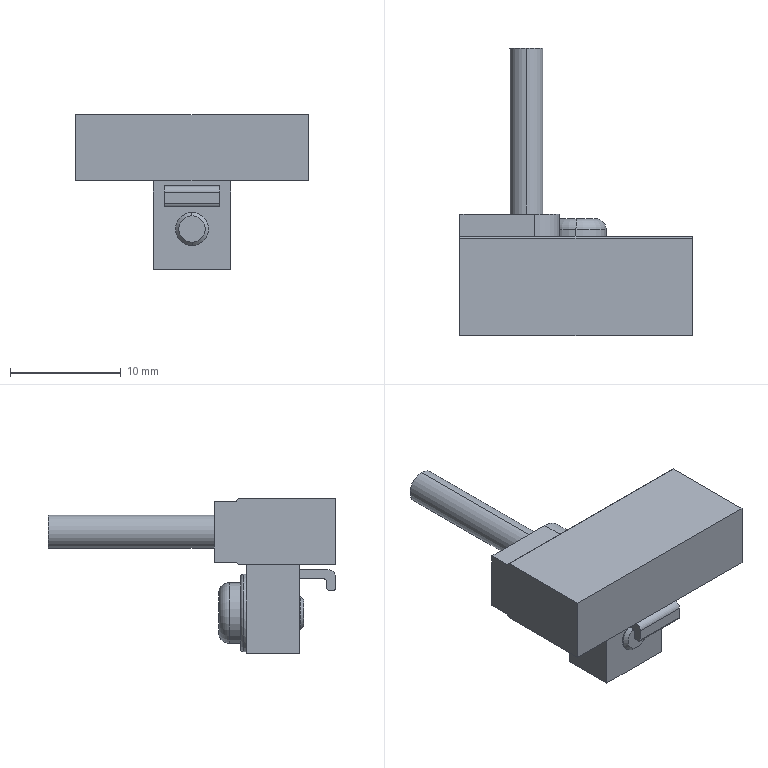Part | SolidWorks | features BaseBody 1 | 1 solid | 49 faces | box 21 x 26 x 14 mm | volume 1685 mm3 | plane 29 | cylinder 14 | torus 4 | cone 2 | commonest cylinder face diameters 3 x4 0.5 x2 4.5 x2 5.5 x2 7 x2 0.6 x1
STEP:
#1=CARTESIAN_POINT('',(10.5,9.6,-4.6));
#2=VERTEX_POINT('',#1);
#3=CARTESIAN_POINT('',(10.5,10.6,-5.6));
#4=VERTEX_POINT('',#3);
#5=CARTESIAN_POINT('',(10.5,9.6,-5.6));
#6=DIRECTION('',(-1.,0.,0.));
#7=DIRECTION('',(0.,0.,1.));
#8=AXIS2_PLACEMENT_3D('',#5,#6,#7);
#9=CIRCLE('',#8,1.);
#10=EDGE_CURVE('',#2,#4,#9,.T.);
#11=ORIENTED_EDGE('',*,*,#10,.F.);
#12=CARTESIAN_POINT('',(10.5,9.6,-10.1));
#13=VERTEX_POINT('',#12);
#14=CARTESIAN_POINT('',(10.5,9.6,-7.35));
#15=DIRECTION('',(0.,1.,0.));
#16=DIRECTION('',(0.,0.,1.));
#17=AXIS2_PLACEMENT_3D('',#14,#15,#16);
#18=CIRCLE('',#17,2.75);
#19=EDGE_CURVE('',#2,#13,#18,.T.);
#20=ORIENTED_EDGE('',*,*,#19,.T.);
#21=CARTESIAN_POINT('',(10.5,10.6,-9.1));
#22=VERTEX_POINT('',#21);
#23=CARTESIAN_POINT('',(10.5,9.6,-9.1));
#24=DIRECTION('',(1.,0.,0.));
#25=DIRECTION('',(0.,0.,-1.));
#26=AXIS2_PLACEMENT_3D('',#23,#24,#25);
#27=CIRCLE('',#26,1.);
#28=EDGE_CURVE('',#13,#22,#27,.T.);
#29=ORIENTED_EDGE('',*,*,#28,.T.);
#30=CARTESIAN_POINT('',(10.5,10.6,-7.35));
#31=DIRECTION('',(0.,1.,0.));
#32=DIRECTION('',(0.,0.,-1.));
#33=AXIS2_PLACEMENT_3D('',#30,#31,#32);
#34=CIRCLE('',#33,1.75);
#35=EDGE_CURVE('',#4,#22,#34,.T.);
#36=ORIENTED_EDGE('',*,*,#35,.F.);
#37=EDGE_LOOP('',(#11,#20,#29,#36));
#38=FACE_OUTER_BOUND('',#37,.T.);
#39=CARTESIAN_POINT('',(10.5,9.6,-7.35));
#40=DIRECTION('',(0.,1.,0.));
#41=DIRECTION('',(0.,0.,-1.));
#42=AXIS2_PLACEMENT_3D('',#39,#40,#41);
#43=TOROIDAL_SURFACE('',#42,1.75,1.);
#44=ADVANCED_FACE('',(#38),#43,.T.);
#45=CARTESIAN_POINT('',(10.5,8.6,-4.6));
#46=VERTEX_POINT('',#45);
#47=CARTESIAN_POINT('',(10.5,10.6,-4.6));
#48=DIRECTION('',(0.,1.,0.));
#49=VECTOR('',#48,1000.);
#50=LINE('',#47,#49);
#51=EDGE_CURVE('',#46,#2,#50,.T.);
#52=ORIENTED_EDGE('',*,*,#51,.F.);
#53=CARTESIAN_POINT('',(10.5,8.6,-10.1));
#54=VERTEX_POINT('',#53);
#55=CARTESIAN_POINT('',(10.5,8.6,-7.35));
#56=DIRECTION('',(0.,1.,0.));
#57=DIRECTION('',(0.,0.,1.));
#58=AXIS2_PLACEMENT_3D('',#55,#56,#57);
#59=CIRCLE('',#58,2.75);
#60=EDGE_CURVE('',#46,#54,#59,.T.);
#61=ORIENTED_EDGE('',*,*,#60,.T.);
#62=CARTESIAN_POINT('',(10.5,10.6,-10.1));
#63=DIRECTION('',(0.,1.,0.));
#64=VECTOR('',#63,1000.);
#65=LINE('',#62,#64);
#66=EDGE_CURVE('',#54,#13,#65,.T.);
#67=ORIENTED_EDGE('',*,*,#66,.T.);
#68=ORIENTED_EDGE('',*,*,#19,.F.);
#69=EDGE_LOOP('',(#52,#61,#67,#68));
#70=FACE_OUTER_BOUND('',#69,.T.);
#71=CARTESIAN_POINT('',(10.5,10.6,-7.35));
#72=DIRECTION('',(0.,1.,0.));
#73=DIRECTION('',(0.000000142,0.,-1.));
#74=AXIS2_PLACEMENT_3D('',#71,#72,#73);
#75=CYLINDRICAL_SURFACE('',#74,2.75);
#76=ADVANCED_FACE('',(#70),#75,.T.);
#77=CARTESIAN_POINT('',(10.5,8.35,-3.85));
#78=VERTEX_POINT('',#77);
#79=CARTESIAN_POINT('',(10.5,8.6,-4.1));
#80=VERTEX_POINT('',#79);
#81=CARTESIAN_POINT('',(10.5,8.35,-4.1));
#82=DIRECTION('',(-1.,0.,-0.000000141));
#83=DIRECTION('',(-0.000000141,0.,1.));
#84=AXIS2_PLACEMENT_3D('',#81,#82,#83);
#85=CIRCLE('',#84,0.25);
#86=EDGE_CURVE('',#78,#80,#85,.T.);
#87=ORIENTED_EDGE('',*,*,#86,.F.);
#88=CARTESIAN_POINT('',(10.5,8.35,-10.85));
#89=VERTEX_POINT('',#88);
#90=CARTESIAN_POINT('',(10.5,8.35,-7.35));
#91=DIRECTION('',(0.,1.,0.));
#92=DIRECTION('',(0.,0.,1.));
#93=AXIS2_PLACEMENT_3D('',#90,#91,#92);
#94=CIRCLE('',#93,3.5);
#95=EDGE_CURVE('',#78,#89,#94,.T.);
#96=ORIENTED_EDGE('',*,*,#95,.T.);
#97=CARTESIAN_POINT('',(10.5,8.6,-10.6));
#98=VERTEX_POINT('',#97);
#99=CARTESIAN_POINT('',(10.5,8.35,-10.6));
#100=DIRECTION('',(1.,0.,0.000000141));
#101=DIRECTION('',(0.000000141,0.,-1.));
#102=AXIS2_PLACEMENT_3D('',#99,#100,#101);
#103=CIRCLE('',#102,0.25);
#104=EDGE_CURVE('',#89,#98,#103,.T.);
#105=ORIENTED_EDGE('',*,*,#104,.T.);
#106=CARTESIAN_POINT('',(10.5,8.6,-7.35));
#107=DIRECTION('',(0.,1.,0.));
#108=DIRECTION('',(0.000000141,0.,-1.));
#109=AXIS2_PLACEMENT_3D('',#106,#107,#108);
#110=CIRCLE('',#109,3.25);
#111=EDGE_CURVE('',#80,#98,#110,.T.);
#112=ORIENTED_EDGE('',*,*,#111,.F.);
#113=EDGE_LOOP('',(#87,#96,#105,#112));
#114=FACE_OUTER_BOUND('',#113,.T.);
#115=CARTESIAN_POINT('',(10.5,8.35,-7.35));
#116=DIRECTION('',(0.,1.,0.));
#117=DIRECTION('',(0.000000141,0.,-1.));
#118=AXIS2_PLACEMENT_3D('',#115,#116,#117);
#119=TOROIDAL_SURFACE('',#118,3.25,0.25);
#120=ADVANCED_FACE('',(#114),#119,.T.);
#121=CARTESIAN_POINT('',(10.5,8.1,-3.85));
#122=VERTEX_POINT('',#121);
#123=CARTESIAN_POINT('',(10.5,10.6,-3.85));
#124=DIRECTION('',(0.,1.,0.));
#125=VECTOR('',#124,1000.);
#126=LINE('',#123,#125);
#127=EDGE_CURVE('',#122,#78,#126,.T.);
#128=ORIENTED_EDGE('',*,*,#127,.F.);
#129=CARTESIAN_POINT('',(14.,8.1,-7.35));
#130=VERTEX_POINT('',#129);
#131=CARTESIAN_POINT('',(10.5,8.1,-7.35));
#132=DIRECTION('',(0.,1.,0.));
#133=DIRECTION('',(0.,0.,1.));
#134=AXIS2_PLACEMENT_3D('',#131,#132,#133);
#135=CIRCLE('',#134,3.5);
#136=EDGE_CURVE('',#122,#130,#135,.T.);
#137=ORIENTED_EDGE('',*,*,#136,.T.);
#138=CARTESIAN_POINT('',(10.5,8.1,-10.85));
#139=VERTEX_POINT('',#138);
#140=CARTESIAN_POINT('',(10.5,8.1,-7.35));
#141=DIRECTION('',(0.,1.,0.));
#142=DIRECTION('',(0.,0.,-1.));
#143=AXIS2_PLACEMENT_3D('',#140,#141,#142);
#144=CIRCLE('',#143,3.5);
#145=EDGE_CURVE('',#130,#139,#144,.T.);
#146=ORIENTED_EDGE('',*,*,#145,.T.);
#147=CARTESIAN_POINT('',(10.5,10.6,-10.85));
#148=DIRECTION('',(0.,1.,0.));
#149=VECTOR('',#148,1000.);
#150=LINE('',#147,#149);
#151=EDGE_CURVE('',#139,#89,#150,.T.);
#152=ORIENTED_EDGE('',*,*,#151,.T.);
#153=ORIENTED_EDGE('',*,*,#95,.F.);
#154=EDGE_LOOP('',(#128,#137,#146,#152,#153));
#155=FACE_OUTER_BOUND('',#154,.T.);
#156=CARTESIAN_POINT('',(10.5,10.6,-7.35));
#157=DIRECTION('',(0.,1.,0.));
#158=DIRECTION('',(0.,0.,-1.));
#159=AXIS2_PLACEMENT_3D('',#156,#157,#158);
#160=CYLINDRICAL_SURFACE('',#159,3.5);
#161=ADVANCED_FACE('',(#155),#160,.T.);
#162=CARTESIAN_POINT('',(10.5,3.207,-5.85));
#163=VERTEX_POINT('',#162);
#164=CARTESIAN_POINT('',(10.5,3.3,-5.85));
#165=VERTEX_POINT('',#164);
#166=CARTESIAN_POINT('',(10.5,10.6,-5.85));
#167=DIRECTION('',(0.,1.,0.));
#168=VECTOR('',#167,1000.);
#169=LINE('',#166,#168);
#170=EDGE_CURVE('',#163,#165,#169,.T.);
#171=ORIENTED_EDGE('',*,*,#170,.F.);
#172=CARTESIAN_POINT('',(10.5,3.207,-8.85));
#173=VERTEX_POINT('',#172);
#174=CARTESIAN_POINT('',(10.5,3.207,-7.35));
#175=DIRECTION('',(0.,1.,0.));
#176=DIRECTION('',(0.,0.,1.));
#177=AXIS2_PLACEMENT_3D('',#174,#175,#176);
#178=CIRCLE('',#177,1.5);
#179=EDGE_CURVE('',#163,#173,#178,.T.);
#180=ORIENTED_EDGE('',*,*,#179,.T.);
#181=CARTESIAN_POINT('',(10.5,3.3,-8.85));
#182=VERTEX_POINT('',#181);
#183=CARTESIAN_POINT('',(10.5,10.6,-8.85));
#184=DIRECTION('',(0.,1.,0.));
#185=VECTOR('',#184,1000.);
#186=LINE('',#183,#185);
#187=EDGE_CURVE('',#173,#182,#186,.T.);
#188=ORIENTED_EDGE('',*,*,#187,.T.);
#189=CARTESIAN_POINT('',(10.5,3.3,-7.35));
#190=DIRECTION('',(0.,-1.,0.));
#191=DIRECTION('',(-0.000000142,0.,-1.));
#192=AXIS2_PLACEMENT_3D('',#189,#190,#191);
#193=CIRCLE('',#192,1.5);
#194=EDGE_CURVE('',#182,#165,#193,.T.);
#195=ORIENTED_EDGE('',*,*,#194,.T.);
#196=EDGE_LOOP('',(#171,#180,#188,#195));
#197=FACE_OUTER_BOUND('',#196,.T.);
#198=CARTESIAN_POINT('',(10.5,10.6,-7.35));
#199=DIRECTION('',(0.,1.,0.));
#200=DIRECTION('',(0.,0.,-1.));
#201=AXIS2_PLACEMENT_3D('',#198,#199,#200);
#202=CYLINDRICAL_SURFACE('',#201,1.5);
#203=ADVANCED_FACE('',(#197),#202,.T.);
#204=CARTESIAN_POINT('',(10.5,2.9,-6.156));
#205=VERTEX_POINT('',#204);
#206=CARTESIAN_POINT('',(10.5,3.207,-5.85));
#207=DIRECTION('',(-0.000000101,0.7071,0.7071));
#208=VECTOR('',#207,1000.);
#209=LINE('',#206,#208);
#210=EDGE_CURVE('',#205,#163,#209,.T.);
#211=ORIENTED_EDGE('',*,*,#210,.F.);
#212=CARTESIAN_POINT('',(10.5,2.9,-8.543));
#213=VERTEX_POINT('',#212);
#214=CARTESIAN_POINT('',(10.5,2.9,-7.35));
#215=DIRECTION('',(0.,1.,0.));
#216=DIRECTION('',(0.,0.,1.));
#217=AXIS2_PLACEMENT_3D('',#214,#215,#216);
#218=CIRCLE('',#217,1.194);
#219=EDGE_CURVE('',#205,#213,#218,.T.);
#220=ORIENTED_EDGE('',*,*,#219,.T.);
#221=CARTESIAN_POINT('',(10.5,3.207,-8.85));
#222=DIRECTION('',(0.000000101,0.7071,-0.7071));
#223=VECTOR('',#222,1000.);
#224=LINE('',#221,#223);
#225=EDGE_CURVE('',#213,#173,#224,.T.);
#226=ORIENTED_EDGE('',*,*,#225,.T.);
#227=ORIENTED_EDGE('',*,*,#179,.F.);
#228=EDGE_LOOP('',(#211,#220,#226,#227));
#229=FACE_OUTER_BOUND('',#228,.T.);
#230=CARTESIAN_POINT('',(10.5,3.207,-7.35));
#231=DIRECTION('',(0.,1.,0.));
#232=DIRECTION('',(0.000000142,0.,-1.));
#233=AXIS2_PLACEMENT_3D('',#230,#231,#232);
#234=CONICAL_SURFACE('',#233,1.5,0.7854);
#235=ADVANCED_FACE('',(#229),#234,.T.);
#236=CARTESIAN_POINT('',(6.,11.,1.5));
#237=VERTEX_POINT('',#236);
#238=CARTESIAN_POINT('',(6.,26.,1.5));
#239=VERTEX_POINT('',#238);
#240=CARTESIAN_POINT('',(6.,26.,1.5));
#241=DIRECTION('',(0.,1.,0.));
#242=VECTOR('',#241,1000.);
#243=LINE('',#240,#242);
#244=EDGE_CURVE('',#237,#239,#243,.T.);
#245=ORIENTED_EDGE('',*,*,#244,.F.);
#246=CARTESIAN_POINT('',(6.,11.,-1.5));
#247=VERTEX_POINT('',#246);
#248=CARTESIAN_POINT('',(6.,11.,0.));
#249=DIRECTION('',(0.,1.,0.));
#250=DIRECTION('',(0.,0.,1.));
#251=AXIS2_PLACEMENT_3D('',#248,#249,#250);
#252=CIRCLE('',#251,1.5);
#253=EDGE_CURVE('',#237,#247,#252,.T.);
#254=ORIENTED_EDGE('',*,*,#253,.T.);
#255=CARTESIAN_POINT('',(6.,26.,-1.5));
#256=VERTEX_POINT('',#255);
#257=CARTESIAN_POINT('',(6.,26.,-1.5));
#258=DIRECTION('',(0.,1.,0.));
#259=VECTOR('',#258,1000.);
#260=LINE('',#257,#259);
#261=EDGE_CURVE('',#247,#256,#260,.T.);
#262=ORIENTED_EDGE('',*,*,#261,.T.);
#263=CARTESIAN_POINT('',(6.,26.,0.));
#264=DIRECTION('',(0.,1.,0.));
#265=DIRECTION('',(0.,0.,-1.));
#266=AXIS2_PLACEMENT_3D('',#263,#264,#265);
#267=CIRCLE('',#266,1.5);
#268=EDGE_CURVE('',#239,#256,#267,.T.);
#269=ORIENTED_EDGE('',*,*,#268,.F.);
#270=EDGE_LOOP('',(#245,#254,#262,#269));
#271=FACE_OUTER_BOUND('',#270,.T.);
#272=CARTESIAN_POINT('',(6.,26.,0.));
#273=DIRECTION('',(0.,1.,0.));
#274=DIRECTION('',(0.,0.,-1.));
#275=AXIS2_PLACEMENT_3D('',#272,#273,#274);
#276=CYLINDRICAL_SURFACE('',#275,1.5);
#277=ADVANCED_FACE('',(#271),#276,.T.);
#278=CARTESIAN_POINT('',(10.5,10.6,-7.35));
#279=DIRECTION('',(0.,1.,0.));
#280=DIRECTION('',(0.,0.,-1.));
#281=AXIS2_PLACEMENT_3D('',#278,#279,#280);
#282=CIRCLE('',#281,1.75);
#283=EDGE_CURVE('',#22,#4,#282,.T.);
#284=ORIENTED_EDGE('',*,*,#283,.T.);
#285=ORIENTED_EDGE('',*,*,#35,.T.);
#286=EDGE_LOOP('',(#284,#285));
#287=FACE_OUTER_BOUND('',#286,.T.);
#288=CARTESIAN_POINT('',(8.75,10.6,-5.6));
#289=DIRECTION('',(0.,1.,0.));
#290=DIRECTION('',(1.,0.,0.));
#291=AXIS2_PLACEMENT_3D('',#288,#289,#290);
#292=PLANE('',#291);
#293=ADVANCED_FACE('',(#287),#292,.T.);
#294=CARTESIAN_POINT('',(10.5,8.6,-7.35));
#295=DIRECTION('',(0.,1.,0.));
#296=DIRECTION('',(0.,0.,1.));
#297=AXIS2_PLACEMENT_3D('',#294,#295,#296);
#298=CIRCLE('',#297,2.75);
#299=EDGE_CURVE('',#54,#46,#298,.T.);
#300=ORIENTED_EDGE('',*,*,#299,.F.);
#301=ORIENTED_EDGE('',*,*,#60,.F.);
#302=EDGE_LOOP('',(#300,#301));
#303=FACE_BOUND('',#302,.T.);
#304=CARTESIAN_POINT('',(10.5,8.6,-7.35));
#305=DIRECTION('',(0.,1.,0.));
#306=DIRECTION('',(0.000000141,0.,-1.));
#307=AXIS2_PLACEMENT_3D('',#304,#305,#306);
#308=CIRCLE('',#307,3.25);
#309=EDGE_CURVE('',#98,#80,#308,.T.);
#310=ORIENTED_EDGE('',*,*,#309,.T.);
#311=ORIENTED_EDGE('',*,*,#111,.T.);
#312=EDGE_LOOP('',(#310,#311));
#313=FACE_OUTER_BOUND('',#312,.T.);
#314=CARTESIAN_POINT('',(7.25,8.6,-4.1));
#315=DIRECTION('',(0.,1.,0.));
#316=DIRECTION('',(1.,0.,0.));
#317=AXIS2_PLACEMENT_3D('',#314,#315,#316);
#318=PLANE('',#317);
#319=ADVANCED_FACE('',(#303,#313),#318,.T.);
#320=CARTESIAN_POINT('',(10.5,2.9,-7.35));
#321=DIRECTION('',(0.,1.,0.));
#322=DIRECTION('',(0.,0.,1.));
#323=AXIS2_PLACEMENT_3D('',#320,#321,#322);
#324=CIRCLE('',#323,1.194);
#325=EDGE_CURVE('',#213,#205,#324,.T.);
#326=ORIENTED_EDGE('',*,*,#325,.F.);
#327=ORIENTED_EDGE('',*,*,#219,.F.);
#328=EDGE_LOOP('',(#326,#327));
#329=FACE_OUTER_BOUND('',#328,.T.);
#330=CARTESIAN_POINT('',(9.291,2.9,-8.544));
#331=DIRECTION('',(0.,-1.,0.));
#332=DIRECTION('',(0.,0.,-1.));
#333=AXIS2_PLACEMENT_3D('',#330,#331,#332);
#334=PLANE('',#333);
#335=ADVANCED_FACE('',(#329),#334,.T.);
#336=CARTESIAN_POINT('',(8.,1.1,-4.25));
#337=VERTEX_POINT('',#336);
#338=CARTESIAN_POINT('',(8.,0.8,-4.55));
#339=VERTEX_POINT('',#338);
#340=CARTESIAN_POINT('',(8.,1.1,-4.55));
#341=DIRECTION('',(1.,0.,0.));
#342=DIRECTION('',(0.,0.,1.));
#343=AXIS2_PLACEMENT_3D('',#340,#341,#342);
#344=CIRCLE('',#343,0.3);
#345=EDGE_CURVE('',#337,#339,#344,.T.);
#346=ORIENTED_EDGE('',*,*,#345,.F.);
#347=CARTESIAN_POINT('',(13.,1.1,-4.25));
#348=VERTEX_POINT('',#347);
#349=CARTESIAN_POINT('',(13.,1.1,-4.25));
#350=DIRECTION('',(-1.,0.,0.));
#351=VECTOR('',#350,1000.);
#352=LINE('',#349,#351);
#353=EDGE_CURVE('',#348,#337,#352,.T.);
#354=ORIENTED_EDGE('',*,*,#353,.F.);
#355=CARTESIAN_POINT('',(13.,0.8,-4.55));
#356=VERTEX_POINT('',#355);
#357=CARTESIAN_POINT('',(13.,1.1,-4.55));
#358=DIRECTION('',(1.,0.,0.));
#359=DIRECTION('',(0.,-1.,0.));
#360=AXIS2_PLACEMENT_3D('',#357,#358,#359);
#361=CIRCLE('',#360,0.3);
#362=EDGE_CURVE('',#348,#356,#361,.T.);
#363=ORIENTED_EDGE('',*,*,#362,.T.);
#364=CARTESIAN_POINT('',(8.,0.8,-4.55));
#365=DIRECTION('',(-1.,0.,0.));
#366=VECTOR('',#365,1000.);
#367=LINE('',#364,#366);
#368=EDGE_CURVE('',#356,#339,#367,.T.);
#369=ORIENTED_EDGE('',*,*,#368,.T.);
#370=EDGE_LOOP('',(#346,#354,#363,#369));
#371=FACE_OUTER_BOUND('',#370,.T.);
#372=CARTESIAN_POINT('',(13.,1.1,-4.55));
#373=DIRECTION('',(-1.,0.,0.));
#374=DIRECTION('',(0.,-1.,0.));
#375=AXIS2_PLACEMENT_3D('',#372,#373,#374);
#376=CYLINDRICAL_SURFACE('',#375,0.3);
#377=ADVANCED_FACE('',(#371),#376,.F.);
#378=CARTESIAN_POINT('',(8.,0.8,-5.07));
#379=VERTEX_POINT('',#378);
#380=CARTESIAN_POINT('',(8.,0.8,-4.55));
#381=DIRECTION('',(0.,0.,1.));
#382=VECTOR('',#381,1000.);
#383=LINE('',#380,#382);
#384=EDGE_CURVE('',#379,#339,#383,.T.);
#385=ORIENTED_EDGE('',*,*,#384,.T.);
#386=ORIENTED_EDGE('',*,*,#368,.F.);
#387=CARTESIAN_POINT('',(13.,0.8,-5.07));
#388=VERTEX_POINT('',#387);
#389=CARTESIAN_POINT('',(13.,0.8,-5.07));
#390=DIRECTION('',(0.,0.,1.));
#391=VECTOR('',#390,1000.);
#392=LINE('',#389,#391);
#393=EDGE_CURVE('',#388,#356,#392,.T.);
#394=ORIENTED_EDGE('',*,*,#393,.F.);
#395=CARTESIAN_POINT('',(8.,0.8,-5.07));
#396=DIRECTION('',(-1.,0.,0.));
#397=VECTOR('',#396,1000.);
#398=LINE('',#395,#397);
#399=EDGE_CURVE('',#388,#379,#398,.T.);
#400=ORIENTED_EDGE('',*,*,#399,.T.);
#401=EDGE_LOOP('',(#385,#386,#394,#400));
#402=FACE_OUTER_BOUND('',#401,.T.);
#403=CARTESIAN_POINT('',(8.,0.8,-4.55));
#404=DIRECTION('',(0.,1.,0.));
#405=DIRECTION('',(1.,0.,0.));
#406=AXIS2_PLACEMENT_3D('',#403,#404,#405);
#407=PLANE('',#406);
#408=ADVANCED_FACE('',(#402),#407,.T.);
#409=CARTESIAN_POINT('',(8.,0.55,-5.32));
#410=VERTEX_POINT('',#409);
#411=CARTESIAN_POINT('',(8.,0.55,-5.07));
#412=DIRECTION('',(1.,0.,0.));
#413=DIRECTION('',(0.,1.,0.));
#414=AXIS2_PLACEMENT_3D('',#411,#412,#413);
#415=CIRCLE('',#414,0.25);
#416=EDGE_CURVE('',#410,#379,#415,.T.);
#417=ORIENTED_EDGE('',*,*,#416,.T.);
#418=ORIENTED_EDGE('',*,*,#399,.F.);
#419=CARTESIAN_POINT('',(13.,0.55,-5.32));
#420=VERTEX_POINT('',#419);
#421=CARTESIAN_POINT('',(13.,0.55,-5.07));
#422=DIRECTION('',(1.,0.,0.));
#423=DIRECTION('',(0.,0.,-1.));
#424=AXIS2_PLACEMENT_3D('',#421,#422,#423);
#425=CIRCLE('',#424,0.25);
#426=EDGE_CURVE('',#420,#388,#425,.T.);
#427=ORIENTED_EDGE('',*,*,#426,.F.);
#428=CARTESIAN_POINT('',(8.,0.55,-5.32));
#429=DIRECTION('',(-1.,0.,0.));
#430=VECTOR('',#429,1000.);
#431=LINE('',#428,#430);
#432=EDGE_CURVE('',#420,#410,#431,.T.);
#433=ORIENTED_EDGE('',*,*,#432,.T.);
#434=EDGE_LOOP('',(#417,#418,#427,#433));
#435=FACE_OUTER_BOUND('',#434,.T.);
#436=CARTESIAN_POINT('',(13.,0.55,-5.07));
#437=DIRECTION('',(-1.,0.,0.));
#438=DIRECTION('',(0.,1.,0.));
#439=AXIS2_PLACEMENT_3D('',#436,#437,#438);
#440=CYLINDRICAL_SURFACE('',#439,0.25);
#441=ADVANCED_FACE('',(#435),#440,.T.);
#442=CARTESIAN_POINT('',(8.,0.25,-5.32));
#443=VERTEX_POINT('',#442);
#444=CARTESIAN_POINT('',(8.,0.55,-5.32));
#445=DIRECTION('',(0.,1.,0.));
#446=VECTOR('',#445,1000.);
#447=LINE('',#444,#446);
#448=EDGE_CURVE('',#443,#410,#447,.T.);
#449=ORIENTED_EDGE('',*,*,#448,.T.);
#450=ORIENTED_EDGE('',*,*,#432,.F.);
#451=CARTESIAN_POINT('',(13.,0.25,-5.32));
#452=VERTEX_POINT('',#451);
#453=CARTESIAN_POINT('',(13.,0.25,-5.32));
#454=DIRECTION('',(0.,1.,0.));
#455=VECTOR('',#454,1000.);
#456=LINE('',#453,#455);
#457=EDGE_CURVE('',#452,#420,#456,.T.);
#458=ORIENTED_EDGE('',*,*,#457,.F.);
#459=CARTESIAN_POINT('',(8.,0.25,-5.32));
#460=DIRECTION('',(-1.,0.,0.));
#461=VECTOR('',#460,1000.);
#462=LINE('',#459,#461);
#463=EDGE_CURVE('',#452,#443,#462,.T.);
#464=ORIENTED_EDGE('',*,*,#463,.T.);
#465=EDGE_LOOP('',(#449,#450,#458,#464));
#466=FACE_OUTER_BOUND('',#465,.T.);
#467=CARTESIAN_POINT('',(8.,0.25,-5.32));
#468=DIRECTION('',(0.,0.,-1.));
#469=DIRECTION('',(0.,-1.,0.));
#470=AXIS2_PLACEMENT_3D('',#467,#468,#469);
#471=PLANE('',#470);
#472=ADVANCED_FACE('',(#466),#471,.T.);
#473=CARTESIAN_POINT('',(8.,0.,-5.07));
#474=VERTEX_POINT('',#473);
#475=CARTESIAN_POINT('',(8.,0.25,-5.07));
#476=DIRECTION('',(1.,0.,0.));
#477=DIRECTION('',(0.,0.,-1.));
#478=AXIS2_PLACEMENT_3D('',#475,#476,#477);
#479=CIRCLE('',#478,0.25);
#480=EDGE_CURVE('',#474,#443,#479,.T.);
#481=ORIENTED_EDGE('',*,*,#480,.T.);
#482=ORIENTED_EDGE('',*,*,#463,.F.);
#483=CARTESIAN_POINT('',(13.,0.,-5.07));
#484=VERTEX_POINT('',#483);
#485=CARTESIAN_POINT('',(13.,0.25,-5.07));
#486=DIRECTION('',(1.,0.,0.));
#487=DIRECTION('',(0.,-1.,0.));
#488=AXIS2_PLACEMENT_3D('',#485,#486,#487);
#489=CIRCLE('',#488,0.25);
#490=EDGE_CURVE('',#484,#452,#489,.T.);
#491=ORIENTED_EDGE('',*,*,#490,.F.);
#492=CARTESIAN_POINT('',(8.,0.,-5.07));
#493=DIRECTION('',(-1.,0.,0.));
#494=VECTOR('',#493,1000.);
#495=LINE('',#492,#494);
#496=EDGE_CURVE('',#484,#474,#495,.T.);
#497=ORIENTED_EDGE('',*,*,#496,.T.);
#498=EDGE_LOOP('',(#481,#482,#491,#497));
#499=FACE_OUTER_BOUND('',#498,.T.);
#500=CARTESIAN_POINT('',(13.,0.25,-5.07));
#501=DIRECTION('',(-1.,0.,0.));
#502=DIRECTION('',(0.,0.,-1.));
#503=AXIS2_PLACEMENT_3D('',#500,#501,#502);
#504=CYLINDRICAL_SURFACE('',#503,0.25);
#505=ADVANCED_FACE('',(#499),#504,.T.);
#506=CARTESIAN_POINT('',(8.,0.,-4.05));
#507=VERTEX_POINT('',#506);
#508=CARTESIAN_POINT('',(8.,0.,-5.07));
#509=DIRECTION('',(0.,0.,-1.));
#510=VECTOR('',#509,1000.);
#511=LINE('',#508,#510);
#512=EDGE_CURVE('',#507,#474,#511,.T.);
#513=ORIENTED_EDGE('',*,*,#512,.T.);
#514=ORIENTED_EDGE('',*,*,#496,.F.);
#515=CARTESIAN_POINT('',(13.,0.,-4.05));
#516=VERTEX_POINT('',#515);
#517=CARTESIAN_POINT('',(13.,0.,-4.05));
#518=DIRECTION('',(0.,0.,-1.));
#519=VECTOR('',#518,1000.);
#520=LINE('',#517,#519);
#521=EDGE_CURVE('',#516,#484,#520,.T.);
#522=ORIENTED_EDGE('',*,*,#521,.F.);
#523=CARTESIAN_POINT('',(8.,0.,-4.05));
#524=DIRECTION('',(-1.,0.,0.));
#525=VECTOR('',#524,1000.);
#526=LINE('',#523,#525);
#527=EDGE_CURVE('',#516,#507,#526,.T.);
#528=ORIENTED_EDGE('',*,*,#527,.T.);
#529=EDGE_LOOP('',(#513,#514,#522,#528));
#530=FACE_OUTER_BOUND('',#529,.T.);
#531=CARTESIAN_POINT('',(8.,0.,-5.07));
#532=DIRECTION('',(0.,-1.,0.));
#533=DIRECTION('',(0.,0.,-1.));
#534=AXIS2_PLACEMENT_3D('',#531,#532,#533);
#535=PLANE('',#534);
#536=ADVANCED_FACE('',(#530),#535,.T.);
#537=CARTESIAN_POINT('',(8.,0.6,-3.45));
#538=VERTEX_POINT('',#537);
#539=CARTESIAN_POINT('',(8.,0.6,-4.05));
#540=DIRECTION('',(1.,0.,0.));
#541=DIRECTION('',(0.,-1.,0.));
#542=AXIS2_PLACEMENT_3D('',#539,#540,#541);
#543=CIRCLE('',#542,0.6);
#544=EDGE_CURVE('',#538,#507,#543,.T.);
#545=ORIENTED_EDGE('',*,*,#544,.T.);
#546=ORIENTED_EDGE('',*,*,#527,.F.);
#547=CARTESIAN_POINT('',(13.,0.6,-3.45));
#548=VERTEX_POINT('',#547);
#549=CARTESIAN_POINT('',(13.,0.6,-4.05));
#550=DIRECTION('',(1.,0.,0.));
#551=DIRECTION('',(0.,0.,1.));
#552=AXIS2_PLACEMENT_3D('',#549,#550,#551);
#553=CIRCLE('',#552,0.6);
#554=EDGE_CURVE('',#548,#516,#553,.T.);
#555=ORIENTED_EDGE('',*,*,#554,.F.);
#556=CARTESIAN_POINT('',(8.,0.6,-3.45));
#557=DIRECTION('',(-1.,0.,0.));
#558=VECTOR('',#557,1000.);
#559=LINE('',#556,#558);
#560=EDGE_CURVE('',#548,#538,#559,.T.);
#561=ORIENTED_EDGE('',*,*,#560,.T.);
#562=EDGE_LOOP('',(#545,#546,#555,#561));
#563=FACE_OUTER_BOUND('',#562,.T.);
#564=CARTESIAN_POINT('',(13.,0.6,-4.05));
#565=DIRECTION('',(-1.,0.,0.));
#566=DIRECTION('',(0.,-1.,0.));
#567=AXIS2_PLACEMENT_3D('',#564,#565,#566);
#568=CYLINDRICAL_SURFACE('',#567,0.6);
#569=ADVANCED_FACE('',(#563),#568,.T.);
#570=CARTESIAN_POINT('',(8.,3.3,-3.45));
#571=VERTEX_POINT('',#570);
#572=CARTESIAN_POINT('',(8.,3.3,-3.45));
#573=DIRECTION('',(0.,-1.,0.));
#574=VECTOR('',#573,1000.);
#575=LINE('',#572,#574);
#576=EDGE_CURVE('',#571,#538,#575,.T.);
#577=ORIENTED_EDGE('',*,*,#576,.F.);
#578=CARTESIAN_POINT('',(8.,3.3,-4.25));
#579=VERTEX_POINT('',#578);
#580=CARTESIAN_POINT('',(8.,3.3,-4.25));
#581=DIRECTION('',(0.,0.,-1.));
#582=VECTOR('',#581,1000.);
#583=LINE('',#580,#582);
#584=EDGE_CURVE('',#571,#579,#583,.T.);
#585=ORIENTED_EDGE('',*,*,#584,.T.);
#586=CARTESIAN_POINT('',(8.,1.1,-4.25));
#587=DIRECTION('',(0.,1.,0.));
#588=VECTOR('',#587,1000.);
#589=LINE('',#586,#588);
#590=EDGE_CURVE('',#337,#579,#589,.T.);
#591=ORIENTED_EDGE('',*,*,#590,.F.);
#592=ORIENTED_EDGE('',*,*,#345,.T.);
#593=ORIENTED_EDGE('',*,*,#384,.F.);
#594=ORIENTED_EDGE('',*,*,#416,.F.);
#595=ORIENTED_EDGE('',*,*,#448,.F.);
#596=ORIENTED_EDGE('',*,*,#480,.F.);
#597=ORIENTED_EDGE('',*,*,#512,.F.);
#598=ORIENTED_EDGE('',*,*,#544,.F.);
#599=EDGE_LOOP('',(#577,#585,#591,#592,#593,#594,#595,#596,#597,#598));
#600=FACE_OUTER_BOUND('',#599,.T.);
#601=CARTESIAN_POINT('',(8.,0.,-3.45));
#602=DIRECTION('',(-1.,0.,0.));
#603=DIRECTION('',(0.,0.,1.));
#604=AXIS2_PLACEMENT_3D('',#601,#602,#603);
#605=PLANE('',#604);
#606=ADVANCED_FACE('',(#600),#605,.T.);
#607=CARTESIAN_POINT('',(13.,3.3,-3.45));
#608=VERTEX_POINT('',#607);
#609=CARTESIAN_POINT('',(13.,3.3,-4.25));
#610=VERTEX_POINT('',#609);
#611=CARTESIAN_POINT('',(13.,3.3,-3.45));
#612=DIRECTION('',(0.,0.,-1.));
#613=VECTOR('',#612,1000.);
#614=LINE('',#611,#613);
#615=EDGE_CURVE('',#608,#610,#614,.T.);
#616=ORIENTED_EDGE('',*,*,#615,.F.);
#617=CARTESIAN_POINT('',(13.,0.6,-3.45));
#618=DIRECTION('',(0.,-1.,0.));
#619=VECTOR('',#618,1000.);
#620=LINE('',#617,#619);
#621=EDGE_CURVE('',#608,#548,#620,.T.);
#622=ORIENTED_EDGE('',*,*,#621,.T.);
#623=ORIENTED_EDGE('',*,*,#554,.T.);
#624=ORIENTED_EDGE('',*,*,#521,.T.);
#625=ORIENTED_EDGE('',*,*,#490,.T.);
#626=ORIENTED_EDGE('',*,*,#457,.T.);
#627=ORIENTED_EDGE('',*,*,#426,.T.);
#628=ORIENTED_EDGE('',*,*,#393,.T.);
#629=ORIENTED_EDGE('',*,*,#362,.F.);
#630=CARTESIAN_POINT('',(13.,3.3,-4.25));
#631=DIRECTION('',(0.,1.,0.));
#632=VECTOR('',#631,1000.);
#633=LINE('',#630,#632);
#634=EDGE_CURVE('',#348,#610,#633,.T.);
#635=ORIENTED_EDGE('',*,*,#634,.T.);
#636=EDGE_LOOP('',(#616,#622,#623,#624,#625,#626,#627,#628,#629,#635));
#637=FACE_OUTER_BOUND('',#636,.T.);
#638=CARTESIAN_POINT('',(13.,0.,-3.45));
#639=DIRECTION('',(1.,0.,0.));
#640=DIRECTION('',(0.,1.,0.));
#641=AXIS2_PLACEMENT_3D('',#638,#639,#640);
#642=PLANE('',#641);
#643=ADVANCED_FACE('',(#637),#642,.T.);
#644=ORIENTED_EDGE('',*,*,#590,.T.);
#645=CARTESIAN_POINT('',(13.,3.3,-4.25));
#646=DIRECTION('',(1.,0.,0.));
#647=VECTOR('',#646,1000.);
#648=LINE('',#645,#647);
#649=EDGE_CURVE('',#579,#610,#648,.T.);
#650=ORIENTED_EDGE('',*,*,#649,.T.);
#651=ORIENTED_EDGE('',*,*,#634,.F.);
#652=ORIENTED_EDGE('',*,*,#353,.T.);
#653=EDGE_LOOP('',(#644,#650,#651,#652));
#654=FACE_OUTER_BOUND('',#653,.T.);
#655=CARTESIAN_POINT('',(8.,1.1,-4.25));
#656=DIRECTION('',(0.,0.,-1.));
#657=DIRECTION('',(0.,-1.,0.));
#658=AXIS2_PLACEMENT_3D('',#655,#656,#657);
#659=PLANE('',#658);
#660=ADVANCED_FACE('',(#654),#659,.T.);
#661=ORIENTED_EDGE('',*,*,#621,.F.);
#662=CARTESIAN_POINT('',(8.,3.3,-3.45));
#663=DIRECTION('',(-1.,0.,0.));
#664=VECTOR('',#663,1000.);
#665=LINE('',#662,#664);
#666=EDGE_CURVE('',#608,#571,#665,.T.);
#667=ORIENTED_EDGE('',*,*,#666,.T.);
#668=ORIENTED_EDGE('',*,*,#576,.T.);
#669=ORIENTED_EDGE('',*,*,#560,.F.);
#670=EDGE_LOOP('',(#661,#667,#668,#669));
#671=FACE_OUTER_BOUND('',#670,.T.);
#672=CARTESIAN_POINT('',(13.,0.6,-3.45));
#673=DIRECTION('',(0.,0.,1.));
#674=DIRECTION('',(1.,0.,0.));
#675=AXIS2_PLACEMENT_3D('',#672,#673,#674);
#676=PLANE('',#675);
#677=ADVANCED_FACE('',(#671),#676,.T.);
#678=CARTESIAN_POINT('',(7.,8.1,-11.));
#679=VERTEX_POINT('',#678);
#680=CARTESIAN_POINT('',(7.,8.1,-7.35));
#681=VERTEX_POINT('',#680);
#682=CARTESIAN_POINT('',(7.,8.1,-11.));
#683=DIRECTION('',(0.,0.,1.));
#684=VECTOR('',#683,1000.);
#685=LINE('',#682,#684);
#686=EDGE_CURVE('',#679,#681,#685,.T.);
#687=ORIENTED_EDGE('',*,*,#686,.F.);
#688=CARTESIAN_POINT('',(7.,3.3,-11.));
#689=VERTEX_POINT('',#688);
#690=CARTESIAN_POINT('',(7.,3.3,-11.));
#691=DIRECTION('',(0.,1.,0.));
#692=VECTOR('',#691,1000.);
#693=LINE('',#690,#692);
#694=EDGE_CURVE('',#689,#679,#693,.T.);
#695=ORIENTED_EDGE('',*,*,#694,.F.);
#696=CARTESIAN_POINT('',(7.,3.3,-3.));
#697=VERTEX_POINT('',#696);
#698=CARTESIAN_POINT('',(7.,3.3,-3.));
#699=DIRECTION('',(0.,0.,-1.));
#700=VECTOR('',#699,1000.);
#701=LINE('',#698,#700);
#702=EDGE_CURVE('',#697,#689,#701,.T.);
#703=ORIENTED_EDGE('',*,*,#702,.F.);
#704=CARTESIAN_POINT('',(7.,8.1,-3.));
#705=VERTEX_POINT('',#704);
#706=CARTESIAN_POINT('',(7.,8.1,-3.));
#707=DIRECTION('',(0.,-1.,0.));
#708=VECTOR('',#707,1000.);
#709=LINE('',#706,#708);
#710=EDGE_CURVE('',#705,#697,#709,.T.);
#711=ORIENTED_EDGE('',*,*,#710,.F.);
#712=CARTESIAN_POINT('',(7.,8.1,-7.35));
#713=DIRECTION('',(0.,0.,1.));
#714=VECTOR('',#713,1000.);
#715=LINE('',#712,#714);
#716=EDGE_CURVE('',#681,#705,#715,.T.);
#717=ORIENTED_EDGE('',*,*,#716,.F.);
#718=EDGE_LOOP('',(#687,#695,#703,#711,#717));
#719=FACE_OUTER_BOUND('',#718,.T.);
#720=CARTESIAN_POINT('',(7.,3.3,-3.));
#721=DIRECTION('',(-1.,0.,0.));
#722=DIRECTION('',(0.,0.,1.));
#723=AXIS2_PLACEMENT_3D('',#720,#721,#722);
#724=PLANE('',#723);
#725=ADVANCED_FACE('',(#719),#724,.T.);
#726=CARTESIAN_POINT('',(14.,8.1,-11.));
#727=VERTEX_POINT('',#726);
#728=CARTESIAN_POINT('',(14.,8.1,-7.35));
#729=DIRECTION('',(0.,0.,1.));
#730=VECTOR('',#729,1000.);
#731=LINE('',#728,#730);
#732=EDGE_CURVE('',#727,#130,#731,.T.);
#733=ORIENTED_EDGE('',*,*,#732,.T.);
#734=CARTESIAN_POINT('',(14.,8.1,-3.));
#735=VERTEX_POINT('',#734);
#736=CARTESIAN_POINT('',(14.,8.1,-3.));
#737=DIRECTION('',(0.,0.,1.));
#738=VECTOR('',#737,1000.);
#739=LINE('',#736,#738);
#740=EDGE_CURVE('',#130,#735,#739,.T.);
#741=ORIENTED_EDGE('',*,*,#740,.T.);
#742=CARTESIAN_POINT('',(14.,3.3,-3.));
#743=VERTEX_POINT('',#742);
#744=CARTESIAN_POINT('',(14.,3.3,-3.));
#745=DIRECTION('',(0.,-1.,0.));
#746=VECTOR('',#745,1000.);
#747=LINE('',#744,#746);
#748=EDGE_CURVE('',#735,#743,#747,.T.);
#749=ORIENTED_EDGE('',*,*,#748,.T.);
#750=CARTESIAN_POINT('',(14.,3.3,-11.));
#751=VERTEX_POINT('',#750);
#752=CARTESIAN_POINT('',(14.,3.3,-11.));
#753=DIRECTION('',(0.,0.,-1.));
#754=VECTOR('',#753,1000.);
#755=LINE('',#752,#754);
#756=EDGE_CURVE('',#743,#751,#755,.T.);
#757=ORIENTED_EDGE('',*,*,#756,.T.);
#758=CARTESIAN_POINT('',(14.,8.1,-11.));
#759=DIRECTION('',(0.,1.,0.));
#760=VECTOR('',#759,1000.);
#761=LINE('',#758,#760);
#762=EDGE_CURVE('',#751,#727,#761,.T.);
#763=ORIENTED_EDGE('',*,*,#762,.T.);
#764=EDGE_LOOP('',(#733,#741,#749,#757,#763));
#765=FACE_OUTER_BOUND('',#764,.T.);
#766=CARTESIAN_POINT('',(14.,3.3,-3.));
#767=DIRECTION('',(1.,0.,0.));
#768=DIRECTION('',(0.,1.,0.));
#769=AXIS2_PLACEMENT_3D('',#766,#767,#768);
#770=PLANE('',#769);
#771=ADVANCED_FACE('',(#765),#770,.T.);
#772=ORIENTED_EDGE('',*,*,#694,.T.);
#773=CARTESIAN_POINT('',(14.,8.1,-11.));
#774=DIRECTION('',(-1.,0.,0.));
#775=VECTOR('',#774,1000.);
#776=LINE('',#773,#775);
#777=EDGE_CURVE('',#727,#679,#776,.T.);
#778=ORIENTED_EDGE('',*,*,#777,.F.);
#779=ORIENTED_EDGE('',*,*,#762,.F.);
#780=CARTESIAN_POINT('',(7.,3.3,-11.));
#781=DIRECTION('',(-1.,0.,0.));
#782=VECTOR('',#781,1000.);
#783=LINE('',#780,#782);
#784=EDGE_CURVE('',#751,#689,#783,.T.);
#785=ORIENTED_EDGE('',*,*,#784,.T.);
#786=EDGE_LOOP('',(#772,#778,#779,#785));
#787=FACE_OUTER_BOUND('',#786,.T.);
#788=CARTESIAN_POINT('',(7.,3.3,-11.));
#789=DIRECTION('',(0.,0.,-1.));
#790=DIRECTION('',(0.,-1.,0.));
#791=AXIS2_PLACEMENT_3D('',#788,#789,#790);
#792=PLANE('',#791);
#793=ADVANCED_FACE('',(#787),#792,.T.);
#794=ORIENTED_EDGE('',*,*,#666,.F.);
#795=ORIENTED_EDGE('',*,*,#615,.T.);
#796=ORIENTED_EDGE('',*,*,#649,.F.);
#797=ORIENTED_EDGE('',*,*,#584,.F.);
#798=EDGE_LOOP('',(#794,#795,#796,#797));
#799=FACE_BOUND('',#798,.T.);
#800=ORIENTED_EDGE('',*,*,#194,.F.);
#801=CARTESIAN_POINT('',(10.5,3.3,-7.35));
#802=DIRECTION('',(0.,-1.,0.));
#803=DIRECTION('',(-0.000000142,0.,-1.));
#804=AXIS2_PLACEMENT_3D('',#801,#802,#803);
#805=CIRCLE('',#804,1.5);
#806=EDGE_CURVE('',#165,#182,#805,.T.);
#807=ORIENTED_EDGE('',*,*,#806,.F.);
#808=EDGE_LOOP('',(#800,#807));
#809=FACE_BOUND('',#808,.T.);
#810=ORIENTED_EDGE('',*,*,#702,.T.);
#811=ORIENTED_EDGE('',*,*,#784,.F.);
#812=ORIENTED_EDGE('',*,*,#756,.F.);
#813=CARTESIAN_POINT('',(7.,3.3,-3.));
#814=DIRECTION('',(-1.,0.,0.));
#815=VECTOR('',#814,1000.);
#816=LINE('',#813,#815);
#817=EDGE_CURVE('',#743,#697,#816,.T.);
#818=ORIENTED_EDGE('',*,*,#817,.T.);
#819=EDGE_LOOP('',(#810,#811,#812,#818));
#820=FACE_OUTER_BOUND('',#819,.T.);
#821=CARTESIAN_POINT('',(7.,3.3,-11.));
#822=DIRECTION('',(0.,-1.,0.));
#823=DIRECTION('',(0.,0.,-1.));
#824=AXIS2_PLACEMENT_3D('',#821,#822,#823);
#825=PLANE('',#824);
#826=ADVANCED_FACE('',(#799,#809,#820),#825,.T.);
#827=ORIENTED_EDGE('',*,*,#145,.F.);
#828=ORIENTED_EDGE('',*,*,#732,.F.);
#829=ORIENTED_EDGE('',*,*,#777,.T.);
#830=ORIENTED_EDGE('',*,*,#686,.T.);
#831=CARTESIAN_POINT('',(10.5,8.1,-7.35));
#832=DIRECTION('',(0.,1.,0.));
#833=DIRECTION('',(0.,0.,-1.));
#834=AXIS2_PLACEMENT_3D('',#831,#832,#833);
#835=CIRCLE('',#834,3.5);
#836=EDGE_CURVE('',#139,#681,#835,.T.);
#837=ORIENTED_EDGE('',*,*,#836,.F.);
#838=EDGE_LOOP('',(#827,#828,#829,#830,#837));
#839=FACE_OUTER_BOUND('',#838,.T.);
#840=CARTESIAN_POINT('',(7.,8.1,-7.35));
#841=DIRECTION('',(0.,1.,0.));
#842=DIRECTION('',(1.,0.,0.));
#843=AXIS2_PLACEMENT_3D('',#840,#841,#842);
#844=PLANE('',#843);
#845=ADVANCED_FACE('',(#839),#844,.T.);
#846=CARTESIAN_POINT('',(6.,26.,0.));
#847=DIRECTION('',(0.,1.,0.));
#848=DIRECTION('',(0.,0.,-1.));
#849=AXIS2_PLACEMENT_3D('',#846,#847,#848);
#850=CIRCLE('',#849,1.5);
#851=EDGE_CURVE('',#256,#239,#850,.T.);
#852=ORIENTED_EDGE('',*,*,#851,.T.);
#853=ORIENTED_EDGE('',*,*,#268,.T.);
#854=EDGE_LOOP('',(#852,#853));
#855=FACE_OUTER_BOUND('',#854,.T.);
#856=CARTESIAN_POINT('',(4.5,26.,1.5));
#857=DIRECTION('',(0.,1.,0.));
#858=DIRECTION('',(1.,0.,0.));
#859=AXIS2_PLACEMENT_3D('',#856,#857,#858);
#860=PLANE('',#859);
#861=ADVANCED_FACE('',(#855),#860,.T.);
#862=CARTESIAN_POINT('',(6.,11.,0.));
#863=DIRECTION('',(0.,1.,0.));
#864=DIRECTION('',(0.,0.,1.));
#865=AXIS2_PLACEMENT_3D('',#862,#863,#864);
#866=CIRCLE('',#865,1.5);
#867=EDGE_CURVE('',#247,#237,#866,.T.);
#868=ORIENTED_EDGE('',*,*,#867,.F.);
#869=ORIENTED_EDGE('',*,*,#253,.F.);
#870=EDGE_LOOP('',(#868,#869));
#871=FACE_BOUND('',#870,.T.);
#872=CARTESIAN_POINT('',(6.75,11.,-2.75));
#873=VERTEX_POINT('',#872);
#874=CARTESIAN_POINT('',(0.,11.,-2.75));
#875=VERTEX_POINT('',#874);
#876=CARTESIAN_POINT('',(0.,11.,-2.75));
#877=DIRECTION('',(-1.,0.,0.));
#878=VECTOR('',#877,1000.);
#879=LINE('',#876,#878);
#880=EDGE_CURVE('',#873,#875,#879,.T.);
#881=ORIENTED_EDGE('',*,*,#880,.T.);
#882=CARTESIAN_POINT('',(0.,11.,2.75));
#883=VERTEX_POINT('',#882);
#884=CARTESIAN_POINT('',(0.,11.,2.75));
#885=DIRECTION('',(0.,0.,1.));
#886=VECTOR('',#885,1000.);
#887=LINE('',#884,#886);
#888=EDGE_CURVE('',#875,#883,#887,.T.);
#889=ORIENTED_EDGE('',*,*,#888,.T.);
#890=CARTESIAN_POINT('',(6.75,11.,2.75));
#891=VERTEX_POINT('',#890);
#892=CARTESIAN_POINT('',(6.75,11.,2.75));
#893=DIRECTION('',(1.,0.,0.));
#894=VECTOR('',#893,1000.);
#895=LINE('',#892,#894);
#896=EDGE_CURVE('',#883,#891,#895,.T.);
#897=ORIENTED_EDGE('',*,*,#896,.T.);
#898=CARTESIAN_POINT('',(9.,11.,0.5));
#899=VERTEX_POINT('',#898);
#900=CARTESIAN_POINT('',(6.75,11.,0.5));
#901=DIRECTION('',(0.,1.,0.));
#902=DIRECTION('',(1.,0.,0.));
#903=AXIS2_PLACEMENT_3D('',#900,#901,#902);
#904=CIRCLE('',#903,2.25);
#905=EDGE_CURVE('',#891,#899,#904,.T.);
#906=ORIENTED_EDGE('',*,*,#905,.T.);
#907=CARTESIAN_POINT('',(9.,11.,-0.5));
#908=VERTEX_POINT('',#907);
#909=CARTESIAN_POINT('',(9.,11.,-0.5));
#910=DIRECTION('',(0.,0.,-1.));
#911=VECTOR('',#910,1000.);
#912=LINE('',#909,#911);
#913=EDGE_CURVE('',#899,#908,#912,.T.);
#914=ORIENTED_EDGE('',*,*,#913,.T.);
#915=CARTESIAN_POINT('',(6.75,11.,-0.5));
#916=DIRECTION('',(0.,1.,0.));
#917=DIRECTION('',(0.,0.,-1.));
#918=AXIS2_PLACEMENT_3D('',#915,#916,#917);
#919=CIRCLE('',#918,2.25);
#920=EDGE_CURVE('',#908,#873,#919,.T.);
#921=ORIENTED_EDGE('',*,*,#920,.T.);
#922=EDGE_LOOP('',(#881,#889,#897,#906,#914,#921));
#923=FACE_OUTER_BOUND('',#922,.T.);
#924=CARTESIAN_POINT('',(0.,11.,-2.75));
#925=DIRECTION('',(0.,1.,0.));
#926=DIRECTION('',(1.,0.,0.));
#927=AXIS2_PLACEMENT_3D('',#924,#925,#926);
#928=PLANE('',#927);
#929=ADVANCED_FACE('',(#871,#923),#928,.T.);
#930=CARTESIAN_POINT('',(9.,9.,-0.5));
#931=VERTEX_POINT('',#930);
#932=CARTESIAN_POINT('',(6.75,9.,-2.75));
#933=VERTEX_POINT('',#932);
#934=CARTESIAN_POINT('',(6.75,9.,-0.5));
#935=DIRECTION('',(0.,1.,0.));
#936=DIRECTION('',(0.,0.,-1.));
#937=AXIS2_PLACEMENT_3D('',#934,#935,#936);
#938=CIRCLE('',#937,2.25);
#939=EDGE_CURVE('',#931,#933,#938,.T.);
#940=ORIENTED_EDGE('',*,*,#939,.T.);
#941=CARTESIAN_POINT('',(6.75,11.,-2.75));
#942=DIRECTION('',(0.,-1.,0.));
#943=VECTOR('',#942,1000.);
#944=LINE('',#941,#943);
#945=EDGE_CURVE('',#873,#933,#944,.T.);
#946=ORIENTED_EDGE('',*,*,#945,.F.);
#947=ORIENTED_EDGE('',*,*,#920,.F.);
#948=CARTESIAN_POINT('',(9.,9.,-0.5));
#949=DIRECTION('',(0.,-1.,0.));
#950=VECTOR('',#949,1000.);
#951=LINE('',#948,#950);
#952=EDGE_CURVE('',#908,#931,#951,.T.);
#953=ORIENTED_EDGE('',*,*,#952,.T.);
#954=EDGE_LOOP('',(#940,#946,#947,#953));
#955=FACE_OUTER_BOUND('',#954,.T.);
#956=CARTESIAN_POINT('',(6.75,11.,-0.5));
#957=DIRECTION('',(0.,-1.,0.));
#958=DIRECTION('',(0.,0.,-1.));
#959=AXIS2_PLACEMENT_3D('',#956,#957,#958);
#960=CYLINDRICAL_SURFACE('',#959,2.25);
#961=ADVANCED_FACE('',(#955),#960,.T.);
#962=CARTESIAN_POINT('',(9.,9.,0.5));
#963=VERTEX_POINT('',#962);
#964=CARTESIAN_POINT('',(9.,9.,-0.5));
#965=DIRECTION('',(0.,0.,-1.));
#966=VECTOR('',#965,1000.);
#967=LINE('',#964,#966);
#968=EDGE_CURVE('',#963,#931,#967,.T.);
#969=ORIENTED_EDGE('',*,*,#968,.T.);
#970=ORIENTED_EDGE('',*,*,#952,.F.);
#971=ORIENTED_EDGE('',*,*,#913,.F.);
#972=CARTESIAN_POINT('',(9.,9.,0.5));
#973=DIRECTION('',(0.,-1.,0.));
#974=VECTOR('',#973,1000.);
#975=LINE('',#972,#974);
#976=EDGE_CURVE('',#899,#963,#975,.T.);
#977=ORIENTED_EDGE('',*,*,#976,.T.);
#978=EDGE_LOOP('',(#969,#970,#971,#977));
#979=FACE_OUTER_BOUND('',#978,.T.);
#980=CARTESIAN_POINT('',(9.,9.,-0.5));
#981=DIRECTION('',(1.,0.,0.));
#982=DIRECTION('',(0.,1.,0.));
#983=AXIS2_PLACEMENT_3D('',#980,#981,#982);
#984=PLANE('',#983);
#985=ADVANCED_FACE('',(#979),#984,.T.);
#986=CARTESIAN_POINT('',(6.75,9.,2.75));
#987=VERTEX_POINT('',#986);
#988=CARTESIAN_POINT('',(6.75,9.,0.5));
#989=DIRECTION('',(0.,1.,0.));
#990=DIRECTION('',(1.,0.,0.));
#991=AXIS2_PLACEMENT_3D('',#988,#989,#990);
#992=CIRCLE('',#991,2.25);
#993=EDGE_CURVE('',#987,#963,#992,.T.);
#994=ORIENTED_EDGE('',*,*,#993,.T.);
#995=ORIENTED_EDGE('',*,*,#976,.F.);
#996=ORIENTED_EDGE('',*,*,#905,.F.);
#997=CARTESIAN_POINT('',(6.75,9.,2.75));
#998=DIRECTION('',(0.,-1.,0.));
#999=VECTOR('',#998,1000.);
#1000=LINE('',#997,#999);
#1001=EDGE_CURVE('',#891,#987,#1000,.T.);
#1002=ORIENTED_EDGE('',*,*,#1001,.T.);
#1003=EDGE_LOOP('',(#994,#995,#996,#1002));
#1004=FACE_OUTER_BOUND('',#1003,.T.);
#1005=CARTESIAN_POINT('',(6.75,11.,0.5));
#1006=DIRECTION('',(0.,-1.,0.));
#1007=DIRECTION('',(1.,0.,0.));
#1008=AXIS2_PLACEMENT_3D('',#1005,#1006,#1007);
#1009=CYLINDRICAL_SURFACE('',#1008,2.25);
#1010=ADVANCED_FACE('',(#1004),#1009,.T.);
#1011=CARTESIAN_POINT('',(0.,9.,2.75));
#1012=VERTEX_POINT('',#1011);
#1013=CARTESIAN_POINT('',(6.75,9.,2.75));
#1014=DIRECTION('',(1.,0.,0.));
#1015=VECTOR('',#1014,1000.);
#1016=LINE('',#1013,#1015);
#1017=EDGE_CURVE('',#1012,#987,#1016,.T.);
#1018=ORIENTED_EDGE('',*,*,#1017,.T.);
#1019=ORIENTED_EDGE('',*,*,#1001,.F.);
#1020=ORIENTED_EDGE('',*,*,#896,.F.);
#1021=CARTESIAN_POINT('',(0.,9.,2.75));
#1022=DIRECTION('',(0.,-1.,0.));
#1023=VECTOR('',#1022,1000.);
#1024=LINE('',#1021,#1023);
#1025=EDGE_CURVE('',#883,#1012,#1024,.T.);
#1026=ORIENTED_EDGE('',*,*,#1025,.T.);
#1027=EDGE_LOOP('',(#1018,#1019,#1020,#1026));
#1028=FACE_OUTER_BOUND('',#1027,.T.);
#1029=CARTESIAN_POINT('',(6.75,9.,2.75));
#1030=DIRECTION('',(0.,0.,1.));
#1031=DIRECTION('',(1.,0.,0.));
#1032=AXIS2_PLACEMENT_3D('',#1029,#1030,#1031);
#1033=PLANE('',#1032);
#1034=ADVANCED_FACE('',(#1028),#1033,.T.);
#1035=CARTESIAN_POINT('',(0.,9.,-2.75));
#1036=VERTEX_POINT('',#1035);
#1037=CARTESIAN_POINT('',(0.,9.,-2.75));
#1038=DIRECTION('',(-1.,0.,0.));
#1039=VECTOR('',#1038,1000.);
#1040=LINE('',#1037,#1039);
#1041=EDGE_CURVE('',#933,#1036,#1040,.T.);
#1042=ORIENTED_EDGE('',*,*,#1041,.T.);
#1043=CARTESIAN_POINT('',(0.,11.,-2.75));
#1044=DIRECTION('',(0.,-1.,0.));
#1045=VECTOR('',#1044,1000.);
#1046=LINE('',#1043,#1045);
#1047=EDGE_CURVE('',#875,#1036,#1046,.T.);
#1048=ORIENTED_EDGE('',*,*,#1047,.F.);
#1049=ORIENTED_EDGE('',*,*,#880,.F.);
#1050=ORIENTED_EDGE('',*,*,#945,.T.);
#1051=EDGE_LOOP('',(#1042,#1048,#1049,#1050));
#1052=FACE_OUTER_BOUND('',#1051,.T.);
#1053=CARTESIAN_POINT('',(0.,9.,-2.75));
#1054=DIRECTION('',(0.,0.,-1.));
#1055=DIRECTION('',(0.,-1.,0.));
#1056=AXIS2_PLACEMENT_3D('',#1053,#1054,#1055);
#1057=PLANE('',#1056);
#1058=ADVANCED_FACE('',(#1052),#1057,.T.);
#1059=CARTESIAN_POINT('',(21.,9.,2.8));
#1060=VERTEX_POINT('',#1059);
#1061=CARTESIAN_POINT('',(21.,8.8,3.));
#1062=VERTEX_POINT('',#1061);
#1063=CARTESIAN_POINT('',(21.,8.8,3.));
#1064=DIRECTION('',(0.,-0.7071,0.7071));
#1065=VECTOR('',#1064,1000.);
#1066=LINE('',#1063,#1065);
#1067=EDGE_CURVE('',#1060,#1062,#1066,.T.);
#1068=ORIENTED_EDGE('',*,*,#1067,.T.);
#1069=CARTESIAN_POINT('',(21.,0.,3.));
#1070=VERTEX_POINT('',#1069);
#1071=CARTESIAN_POINT('',(21.,0.,3.));
#1072=DIRECTION('',(0.,-1.,0.));
#1073=VECTOR('',#1072,1000.);
#1074=LINE('',#1071,#1073);
#1075=EDGE_CURVE('',#1062,#1070,#1074,.T.);
#1076=ORIENTED_EDGE('',*,*,#1075,.T.);
#1077=CARTESIAN_POINT('',(21.,0.,-3.));
#1078=VERTEX_POINT('',#1077);
#1079=CARTESIAN_POINT('',(21.,0.,-3.));
#1080=DIRECTION('',(0.,0.,-1.));
#1081=VECTOR('',#1080,1000.);
#1082=LINE('',#1079,#1081);
#1083=EDGE_CURVE('',#1070,#1078,#1082,.T.);
#1084=ORIENTED_EDGE('',*,*,#1083,.T.);
#1085=CARTESIAN_POINT('',(21.,8.8,-3.));
#1086=VERTEX_POINT('',#1085);
#1087=CARTESIAN_POINT('',(21.,8.8,-3.));
#1088=DIRECTION('',(0.,1.,0.));
#1089=VECTOR('',#1088,1000.);
#1090=LINE('',#1087,#1089);
#1091=EDGE_CURVE('',#1078,#1086,#1090,.T.);
#1092=ORIENTED_EDGE('',*,*,#1091,.T.);
#1093=CARTESIAN_POINT('',(21.,9.,-2.8));
#1094=VERTEX_POINT('',#1093);
#1095=CARTESIAN_POINT('',(21.,9.,-2.8));
#1096=DIRECTION('',(0.,0.7071,0.7071));
#1097=VECTOR('',#1096,1000.);
#1098=LINE('',#1095,#1097);
#1099=EDGE_CURVE('',#1086,#1094,#1098,.T.);
#1100=ORIENTED_EDGE('',*,*,#1099,.T.);
#1101=CARTESIAN_POINT('',(21.,9.,2.8));
#1102=DIRECTION('',(0.,0.,1.));
#1103=VECTOR('',#1102,1000.);
#1104=LINE('',#1101,#1103);
#1105=EDGE_CURVE('',#1094,#1060,#1104,.T.);
#1106=ORIENTED_EDGE('',*,*,#1105,.T.);
#1107=EDGE_LOOP('',(#1068,#1076,#1084,#1092,#1100,#1106));
#1108=FACE_OUTER_BOUND('',#1107,.T.);
#1109=CARTESIAN_POINT('',(21.,0.,-3.));
#1110=DIRECTION('',(1.,0.,0.));
#1111=DIRECTION('',(0.,1.,0.));
#1112=AXIS2_PLACEMENT_3D('',#1109,#1110,#1111);
#1113=PLANE('',#1112);
#1114=ADVANCED_FACE('',(#1108),#1113,.T.);
#1115=CARTESIAN_POINT('',(0.,9.,2.8));
#1116=VERTEX_POINT('',#1115);
#1117=CARTESIAN_POINT('',(0.,8.8,3.));
#1118=VERTEX_POINT('',#1117);
#1119=CARTESIAN_POINT('',(0.,9.,2.8));
#1120=DIRECTION('',(0.,-0.7071,0.7071));
#1121=VECTOR('',#1120,1000.);
#1122=LINE('',#1119,#1121);
#1123=EDGE_CURVE('',#1116,#1118,#1122,.T.);
#1124=ORIENTED_EDGE('',*,*,#1123,.F.);
#1125=CARTESIAN_POINT('',(0.,9.,2.75));
#1126=DIRECTION('',(0.,0.,1.));
#1127=VECTOR('',#1126,1000.);
#1128=LINE('',#1125,#1127);
#1129=EDGE_CURVE('',#1012,#1116,#1128,.T.);
#1130=ORIENTED_EDGE('',*,*,#1129,.F.);
#1131=ORIENTED_EDGE('',*,*,#1025,.F.);
#1132=ORIENTED_EDGE('',*,*,#888,.F.);
#1133=ORIENTED_EDGE('',*,*,#1047,.T.);
#1134=CARTESIAN_POINT('',(0.,9.,-2.8));
#1135=VERTEX_POINT('',#1134);
#1136=CARTESIAN_POINT('',(0.,9.,-2.8));
#1137=DIRECTION('',(0.,0.,1.));
#1138=VECTOR('',#1137,1000.);
#1139=LINE('',#1136,#1138);
#1140=EDGE_CURVE('',#1135,#1036,#1139,.T.);
#1141=ORIENTED_EDGE('',*,*,#1140,.F.);
#1142=CARTESIAN_POINT('',(0.,8.8,-3.));
#1143=VERTEX_POINT('',#1142);
#1144=CARTESIAN_POINT('',(0.,8.8,-3.));
#1145=DIRECTION('',(0.,0.7071,0.7071));
#1146=VECTOR('',#1145,1000.);
#1147=LINE('',#1144,#1146);
#1148=EDGE_CURVE('',#1143,#1135,#1147,.T.);
#1149=ORIENTED_EDGE('',*,*,#1148,.F.);
#1150=CARTESIAN_POINT('',(0.,0.,-3.));
#1151=VERTEX_POINT('',#1150);
#1152=CARTESIAN_POINT('',(0.,0.,-3.));
#1153=DIRECTION('',(0.,1.,0.));
#1154=VECTOR('',#1153,1000.);
#1155=LINE('',#1152,#1154);
#1156=EDGE_CURVE('',#1151,#1143,#1155,.T.);
#1157=ORIENTED_EDGE('',*,*,#1156,.F.);
#1158=CARTESIAN_POINT('',(0.,0.,3.));
#1159=VERTEX_POINT('',#1158);
#1160=CARTESIAN_POINT('',(0.,0.,3.));
#1161=DIRECTION('',(0.,0.,-1.));
#1162=VECTOR('',#1161,1000.);
#1163=LINE('',#1160,#1162);
#1164=EDGE_CURVE('',#1159,#1151,#1163,.T.);
#1165=ORIENTED_EDGE('',*,*,#1164,.F.);
#1166=CARTESIAN_POINT('',(0.,8.8,3.));
#1167=DIRECTION('',(0.,-1.,0.));
#1168=VECTOR('',#1167,1000.);
#1169=LINE('',#1166,#1168);
#1170=EDGE_CURVE('',#1118,#1159,#1169,.T.);
#1171=ORIENTED_EDGE('',*,*,#1170,.F.);
#1172=EDGE_LOOP('',(#1124,#1130,#1131,#1132,#1133,#1141,#1149,#1157,#1165,#1171));
#1173=FACE_OUTER_BOUND('',#1172,.T.);
#1174=CARTESIAN_POINT('',(0.,0.,-3.));
#1175=DIRECTION('',(-1.,0.,0.));
#1176=DIRECTION('',(0.,0.,1.));
#1177=AXIS2_PLACEMENT_3D('',#1174,#1175,#1176);
#1178=PLANE('',#1177);
#1179=ADVANCED_FACE('',(#1173),#1178,.T.);
#1180=ORIENTED_EDGE('',*,*,#1041,.F.);
#1181=ORIENTED_EDGE('',*,*,#939,.F.);
#1182=ORIENTED_EDGE('',*,*,#968,.F.);
#1183=ORIENTED_EDGE('',*,*,#993,.F.);
#1184=ORIENTED_EDGE('',*,*,#1017,.F.);
#1185=ORIENTED_EDGE('',*,*,#1129,.T.);
#1186=CARTESIAN_POINT('',(21.,9.,2.8));
#1187=DIRECTION('',(1.,0.,0.));
#1188=VECTOR('',#1187,1000.);
#1189=LINE('',#1186,#1188);
#1190=EDGE_CURVE('',#1116,#1060,#1189,.T.);
#1191=ORIENTED_EDGE('',*,*,#1190,.T.);
#1192=ORIENTED_EDGE('',*,*,#1105,.F.);
#1193=CARTESIAN_POINT('',(0.,9.,-2.8));
#1194=DIRECTION('',(1.,0.,0.));
#1195=VECTOR('',#1194,1000.);
#1196=LINE('',#1193,#1195);
#1197=EDGE_CURVE('',#1135,#1094,#1196,.T.);
#1198=ORIENTED_EDGE('',*,*,#1197,.F.);
#1199=ORIENTED_EDGE('',*,*,#1140,.T.);
#1200=EDGE_LOOP('',(#1180,#1181,#1182,#1183,#1184,#1185,#1191,#1192,#1198,#1199));
#1201=FACE_OUTER_BOUND('',#1200,.T.);
#1202=CARTESIAN_POINT('',(0.,9.,-2.8));
#1203=DIRECTION('',(0.,1.,0.));
#1204=DIRECTION('',(1.,0.,0.));
#1205=AXIS2_PLACEMENT_3D('',#1202,#1203,#1204);
#1206=PLANE('',#1205);
#1207=ADVANCED_FACE('',(#1201),#1206,.T.);
#1208=ORIENTED_EDGE('',*,*,#1099,.F.);
#1209=CARTESIAN_POINT('',(0.,8.8,-3.));
#1210=DIRECTION('',(1.,0.,0.));
#1211=VECTOR('',#1210,1000.);
#1212=LINE('',#1209,#1211);
#1213=EDGE_CURVE('',#1143,#1086,#1212,.T.);
#1214=ORIENTED_EDGE('',*,*,#1213,.F.);
#1215=ORIENTED_EDGE('',*,*,#1148,.T.);
#1216=ORIENTED_EDGE('',*,*,#1197,.T.);
#1217=EDGE_LOOP('',(#1208,#1214,#1215,#1216));
#1218=FACE_OUTER_BOUND('',#1217,.T.);
#1219=CARTESIAN_POINT('',(0.,8.8,-3.));
#1220=DIRECTION('',(0.,0.7071,-0.7071));
#1221=DIRECTION('',(-1.,0.,0.));
#1222=AXIS2_PLACEMENT_3D('',#1219,#1220,#1221);
#1223=PLANE('',#1222);
#1224=ADVANCED_FACE('',(#1218),#1223,.T.);
#1225=ORIENTED_EDGE('',*,*,#1083,.F.);
#1226=CARTESIAN_POINT('',(0.,0.,3.));
#1227=DIRECTION('',(1.,0.,0.));
#1228=VECTOR('',#1227,1000.);
#1229=LINE('',#1226,#1228);
#1230=EDGE_CURVE('',#1159,#1070,#1229,.T.);
#1231=ORIENTED_EDGE('',*,*,#1230,.F.);
#1232=ORIENTED_EDGE('',*,*,#1164,.T.);
#1233=CARTESIAN_POINT('',(21.,0.,-3.));
#1234=DIRECTION('',(1.,0.,0.));
#1235=VECTOR('',#1234,1000.);
#1236=LINE('',#1233,#1235);
#1237=EDGE_CURVE('',#1151,#1078,#1236,.T.);
#1238=ORIENTED_EDGE('',*,*,#1237,.T.);
#1239=EDGE_LOOP('',(#1225,#1231,#1232,#1238));
#1240=FACE_OUTER_BOUND('',#1239,.T.);
#1241=CARTESIAN_POINT('',(0.,0.,3.));
#1242=DIRECTION('',(0.,-1.,0.));
#1243=DIRECTION('',(0.,0.,-1.));
#1244=AXIS2_PLACEMENT_3D('',#1241,#1242,#1243);
#1245=PLANE('',#1244);
#1246=ADVANCED_FACE('',(#1240),#1245,.T.);
#1247=ORIENTED_EDGE('',*,*,#1075,.F.);
#1248=CARTESIAN_POINT('',(0.,8.8,3.));
#1249=DIRECTION('',(1.,0.,0.));
#1250=VECTOR('',#1249,1000.);
#1251=LINE('',#1248,#1250);
#1252=EDGE_CURVE('',#1118,#1062,#1251,.T.);
#1253=ORIENTED_EDGE('',*,*,#1252,.F.);
#1254=ORIENTED_EDGE('',*,*,#1170,.T.);
#1255=ORIENTED_EDGE('',*,*,#1230,.T.);
#1256=EDGE_LOOP('',(#1247,#1253,#1254,#1255));
#1257=FACE_OUTER_BOUND('',#1256,.T.);
#1258=CARTESIAN_POINT('',(0.,0.,3.));
#1259=DIRECTION('',(0.,0.,1.));
#1260=DIRECTION('',(1.,0.,0.));
#1261=AXIS2_PLACEMENT_3D('',#1258,#1259,#1260);
#1262=PLANE('',#1261);
#1263=ADVANCED_FACE('',(#1257),#1262,.T.);
#1264=ORIENTED_EDGE('',*,*,#1067,.F.);
#1265=ORIENTED_EDGE('',*,*,#1190,.F.);
#1266=ORIENTED_EDGE('',*,*,#1123,.T.);
#1267=ORIENTED_EDGE('',*,*,#1252,.T.);
#1268=EDGE_LOOP('',(#1264,#1265,#1266,#1267));
#1269=FACE_OUTER_BOUND('',#1268,.T.);
#1270=CARTESIAN_POINT('',(0.,9.,2.8));
#1271=DIRECTION('',(0.,0.7071,0.7071));
#1272=DIRECTION('',(1.,0.,0.));
#1273=AXIS2_PLACEMENT_3D('',#1270,#1271,#1272);
#1274=PLANE('',#1273);
#1275=ADVANCED_FACE('',(#1269),#1274,.T.);
#1276=CARTESIAN_POINT('',(7.,8.1,-3.));
#1277=DIRECTION('',(-1.,0.,0.));
#1278=VECTOR('',#1277,1000.);
#1279=LINE('',#1276,#1278);
#1280=EDGE_CURVE('',#735,#705,#1279,.T.);
#1281=ORIENTED_EDGE('',*,*,#1280,.T.);
#1282=ORIENTED_EDGE('',*,*,#710,.T.);
#1283=ORIENTED_EDGE('',*,*,#817,.F.);
#1284=ORIENTED_EDGE('',*,*,#748,.F.);
#1285=EDGE_LOOP('',(#1281,#1282,#1283,#1284));
#1286=FACE_BOUND('',#1285,.T.);
#1287=ORIENTED_EDGE('',*,*,#1091,.F.);
#1288=ORIENTED_EDGE('',*,*,#1237,.F.);
#1289=ORIENTED_EDGE('',*,*,#1156,.T.);
#1290=ORIENTED_EDGE('',*,*,#1213,.T.);
#1291=EDGE_LOOP('',(#1287,#1288,#1289,#1290));
#1292=FACE_OUTER_BOUND('',#1291,.T.);
#1293=CARTESIAN_POINT('',(21.,0.,-3.));
#1294=DIRECTION('',(0.,0.,-1.));
#1295=DIRECTION('',(0.,-1.,0.));
#1296=AXIS2_PLACEMENT_3D('',#1293,#1294,#1295);
#1297=PLANE('',#1296);
#1298=ADVANCED_FACE('',(#1286,#1292),#1297,.T.);
#1299=CARTESIAN_POINT('',(10.5,8.1,-7.35));
#1300=DIRECTION('',(0.,1.,0.));
#1301=DIRECTION('',(0.,0.,1.));
#1302=AXIS2_PLACEMENT_3D('',#1299,#1300,#1301);
#1303=CIRCLE('',#1302,3.5);
#1304=EDGE_CURVE('',#681,#122,#1303,.T.);
#1305=ORIENTED_EDGE('',*,*,#1304,.F.);
#1306=ORIENTED_EDGE('',*,*,#716,.T.);
#1307=ORIENTED_EDGE('',*,*,#1280,.F.);
#1308=ORIENTED_EDGE('',*,*,#740,.F.);
#1309=ORIENTED_EDGE('',*,*,#136,.F.);
#1310=EDGE_LOOP('',(#1305,#1306,#1307,#1308,#1309));
#1311=FACE_OUTER_BOUND('',#1310,.T.);
#1312=CARTESIAN_POINT('',(7.,8.1,-3.));
#1313=DIRECTION('',(0.,1.,0.));
#1314=DIRECTION('',(1.,0.,0.));
#1315=AXIS2_PLACEMENT_3D('',#1312,#1313,#1314);
#1316=PLANE('',#1315);
#1317=ADVANCED_FACE('',(#1311),#1316,.T.);
#1318=ORIENTED_EDGE('',*,*,#867,.T.);
#1319=ORIENTED_EDGE('',*,*,#244,.T.);
#1320=ORIENTED_EDGE('',*,*,#851,.F.);
#1321=ORIENTED_EDGE('',*,*,#261,.F.);
#1322=EDGE_LOOP('',(#1318,#1319,#1320,#1321));
#1323=FACE_OUTER_BOUND('',#1322,.T.);
#1324=CARTESIAN_POINT('',(6.,26.,0.));
#1325=DIRECTION('',(0.,1.,0.));
#1326=DIRECTION('',(0.,0.,-1.));
#1327=AXIS2_PLACEMENT_3D('',#1324,#1325,#1326);
#1328=CYLINDRICAL_SURFACE('',#1327,1.5);
#1329=ADVANCED_FACE('',(#1323),#1328,.T.);
#1330=ORIENTED_EDGE('',*,*,#325,.T.);
#1331=ORIENTED_EDGE('',*,*,#210,.T.);
#1332=CARTESIAN_POINT('',(10.5,3.207,-7.35));
#1333=DIRECTION('',(0.,1.,0.));
#1334=DIRECTION('',(0.,0.,1.));
#1335=AXIS2_PLACEMENT_3D('',#1332,#1333,#1334);
#1336=CIRCLE('',#1335,1.5);
#1337=EDGE_CURVE('',#173,#163,#1336,.T.);
#1338=ORIENTED_EDGE('',*,*,#1337,.F.);
#1339=ORIENTED_EDGE('',*,*,#225,.F.);
#1340=EDGE_LOOP('',(#1330,#1331,#1338,#1339));
#1341=FACE_OUTER_BOUND('',#1340,.T.);
#1342=CARTESIAN_POINT('',(10.5,3.207,-7.35));
#1343=DIRECTION('',(0.,1.,0.));
#1344=DIRECTION('',(0.000000142,0.,-1.));
#1345=AXIS2_PLACEMENT_3D('',#1342,#1343,#1344);
#1346=CONICAL_SURFACE('',#1345,1.5,0.7854);
#1347=ADVANCED_FACE('',(#1341),#1346,.T.);
#1348=ORIENTED_EDGE('',*,*,#1337,.T.);
#1349=ORIENTED_EDGE('',*,*,#170,.T.);
#1350=ORIENTED_EDGE('',*,*,#806,.T.);
#1351=ORIENTED_EDGE('',*,*,#187,.F.);
#1352=EDGE_LOOP('',(#1348,#1349,#1350,#1351));
#1353=FACE_OUTER_BOUND('',#1352,.T.);
#1354=CARTESIAN_POINT('',(10.5,10.6,-7.35));
#1355=DIRECTION('',(0.,1.,0.));
#1356=DIRECTION('',(0.,0.,-1.));
#1357=AXIS2_PLACEMENT_3D('',#1354,#1355,#1356);
#1358=CYLINDRICAL_SURFACE('',#1357,1.5);
#1359=ADVANCED_FACE('',(#1353),#1358,.T.);
#1360=ORIENTED_EDGE('',*,*,#1304,.T.);
#1361=ORIENTED_EDGE('',*,*,#127,.T.);
#1362=CARTESIAN_POINT('',(10.5,8.35,-7.35));
#1363=DIRECTION('',(0.,1.,0.));
#1364=DIRECTION('',(0.,0.,1.));
#1365=AXIS2_PLACEMENT_3D('',#1362,#1363,#1364);
#1366=CIRCLE('',#1365,3.5);
#1367=EDGE_CURVE('',#89,#78,#1366,.T.);
#1368=ORIENTED_EDGE('',*,*,#1367,.F.);
#1369=ORIENTED_EDGE('',*,*,#151,.F.);
#1370=ORIENTED_EDGE('',*,*,#836,.T.);
#1371=EDGE_LOOP('',(#1360,#1361,#1368,#1369,#1370));
#1372=FACE_OUTER_BOUND('',#1371,.T.);
#1373=CARTESIAN_POINT('',(10.5,10.6,-7.35));
#1374=DIRECTION('',(0.,1.,0.));
#1375=DIRECTION('',(0.,0.,-1.));
#1376=AXIS2_PLACEMENT_3D('',#1373,#1374,#1375);
#1377=CYLINDRICAL_SURFACE('',#1376,3.5);
#1378=ADVANCED_FACE('',(#1372),#1377,.T.);
#1379=ORIENTED_EDGE('',*,*,#1367,.T.);
#1380=ORIENTED_EDGE('',*,*,#86,.T.);
#1381=ORIENTED_EDGE('',*,*,#309,.F.);
#1382=ORIENTED_EDGE('',*,*,#104,.F.);
#1383=EDGE_LOOP('',(#1379,#1380,#1381,#1382));
#1384=FACE_OUTER_BOUND('',#1383,.T.);
#1385=CARTESIAN_POINT('',(10.5,8.35,-7.35));
#1386=DIRECTION('',(0.,1.,0.));
#1387=DIRECTION('',(0.000000141,0.,-1.));
#1388=AXIS2_PLACEMENT_3D('',#1385,#1386,#1387);
#1389=TOROIDAL_SURFACE('',#1388,3.25,0.25);
#1390=ADVANCED_FACE('',(#1384),#1389,.T.);
#1391=ORIENTED_EDGE('',*,*,#299,.T.);
#1392=ORIENTED_EDGE('',*,*,#51,.T.);
#1393=CARTESIAN_POINT('',(10.5,9.6,-7.35));
#1394=DIRECTION('',(0.,1.,0.));
#1395=DIRECTION('',(0.,0.,1.));
#1396=AXIS2_PLACEMENT_3D('',#1393,#1394,#1395);
#1397=CIRCLE('',#1396,2.75);
#1398=EDGE_CURVE('',#13,#2,#1397,.T.);
#1399=ORIENTED_EDGE('',*,*,#1398,.F.);
#1400=ORIENTED_EDGE('',*,*,#66,.F.);
#1401=EDGE_LOOP('',(#1391,#1392,#1399,#1400));
#1402=FACE_OUTER_BOUND('',#1401,.T.);
#1403=CARTESIAN_POINT('',(10.5,10.6,-7.35));
#1404=DIRECTION('',(0.,1.,0.));
#1405=DIRECTION('',(0.000000142,0.,-1.));
#1406=AXIS2_PLACEMENT_3D('',#1403,#1404,#1405);
#1407=CYLINDRICAL_SURFACE('',#1406,2.75);
#1408=ADVANCED_FACE('',(#1402),#1407,.T.);
#1409=ORIENTED_EDGE('',*,*,#1398,.T.);
#1410=ORIENTED_EDGE('',*,*,#10,.T.);
#1411=ORIENTED_EDGE('',*,*,#283,.F.);
#1412=ORIENTED_EDGE('',*,*,#28,.F.);
#1413=EDGE_LOOP('',(#1409,#1410,#1411,#1412));
#1414=FACE_OUTER_BOUND('',#1413,.T.);
#1415=CARTESIAN_POINT('',(10.5,9.6,-7.35));
#1416=DIRECTION('',(0.,1.,0.));
#1417=DIRECTION('',(0.,0.,-1.));
#1418=AXIS2_PLACEMENT_3D('',#1415,#1416,#1417);
#1419=TOROIDAL_SURFACE('',#1418,1.75,1.);
#1420=ADVANCED_FACE('',(#1414),#1419,.T.);
#1421=CLOSED_SHELL('',(#44,#76,#120,#161,#203,#235,#277,#293,#319,#335,#377,#408,#441,#472,#505,#536,#569,#606,#643,#660,#677,#725,#771,#793,#826,#845,#861,#929,#961,#985,#1010,#1034,#1058,#1114,#1179,#1207,#1224,#1246,#1263,#1275,#1298,#1317,#1329,#1347,#1359,#1378,#1390,#1408,#1420));
#1422=MANIFOLD_SOLID_BREP('',#1421);
#1423=CARTESIAN_POINT('',(0.,0.,0.));
#1424=DIRECTION('',(0.,0.,1.));
#1425=DIRECTION('',(1.,0.,0.));
#1426=AXIS2_PLACEMENT_3D('',#1423,#1424,#1425);
#1427=(LENGTH_UNIT()NAMED_UNIT(*)SI_UNIT(.MILLI.,.METRE.));
#1428=UNCERTAINTY_MEASURE_WITH_UNIT(LENGTH_MEASURE(0.00001),#1427,'','');
#1429=(NAMED_UNIT(*)PLANE_ANGLE_UNIT()SI_UNIT($,.RADIAN.));
#1430=(NAMED_UNIT(*)SI_UNIT($,.STERADIAN.)SOLID_ANGLE_UNIT());
#1431=(GEOMETRIC_REPRESENTATION_CONTEXT(3)GLOBAL_UNCERTAINTY_ASSIGNED_CONTEXT((#1428))GLOBAL_UNIT_ASSIGNED_CONTEXT((#1427,#1429,#1430))REPRESENTATION_CONTEXT('',''));
#1432=ADVANCED_BREP_SHAPE_REPRESENTATION('',(#1422,#1426),#1431);